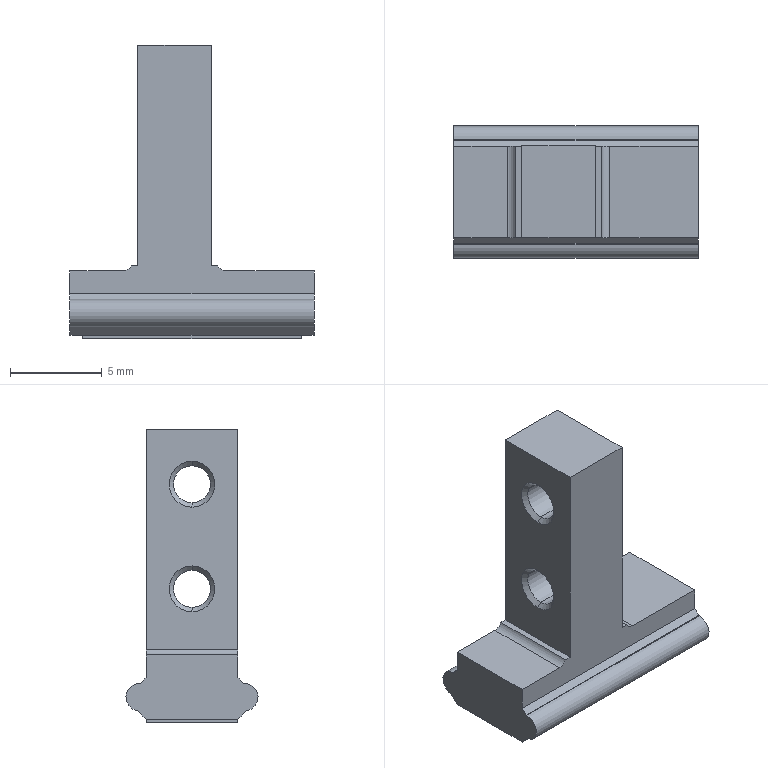Part | SolidWorks | features ICE 5, Chamfer 3, HoleWzd 2, Cut 1, Extrusion 1 | 1 solid | 43 faces | box 13.3 x 7.2 x 16 mm | volume 492.464 mm3 | plane 23 | cylinder 12 | cone 8 | commonest cylinder face diameters 1.5 x4 2.013 x4 1 x2 2.5 x2
STEP:
#1=CARTESIAN_POINT('',(-8.85,0.,3.));
#2=VERTEX_POINT('',#1);
#3=CARTESIAN_POINT('',(-11.35,0.,3.));
#4=VERTEX_POINT('',#3);
#5=CARTESIAN_POINT('',(-10.1,0.,3.));
#6=DIRECTION('',(0.,0.,-1.));
#7=DIRECTION('',(-1.,0.,0.));
#8=AXIS2_PLACEMENT_3D('',#5,#6,#7);
#9=CIRCLE('',#8,1.25);
#10=EDGE_CURVE('',#2,#4,#9,.T.);
#11=ORIENTED_EDGE('',*,*,#10,.F.);
#12=CARTESIAN_POINT('',(-8.85,0.,0.));
#13=VERTEX_POINT('',#12);
#14=CARTESIAN_POINT('',(-8.85,0.,3.));
#15=DIRECTION('',(0.,0.,-1.));
#16=VECTOR('',#15,1000.);
#17=LINE('',#14,#16);
#18=EDGE_CURVE('',#2,#13,#17,.T.);
#19=ORIENTED_EDGE('',*,*,#18,.T.);
#20=CARTESIAN_POINT('',(-11.35,0.,0.));
#21=VERTEX_POINT('',#20);
#22=CARTESIAN_POINT('',(-10.1,0.,0.));
#23=DIRECTION('',(0.,0.,-1.));
#24=DIRECTION('',(-1.,0.,0.));
#25=AXIS2_PLACEMENT_3D('',#22,#23,#24);
#26=CIRCLE('',#25,1.25);
#27=EDGE_CURVE('',#13,#21,#26,.T.);
#28=ORIENTED_EDGE('',*,*,#27,.T.);
#29=CARTESIAN_POINT('',(-11.35,0.,3.));
#30=DIRECTION('',(0.,0.,-1.));
#31=VECTOR('',#30,1000.);
#32=LINE('',#29,#31);
#33=EDGE_CURVE('',#4,#21,#32,.T.);
#34=ORIENTED_EDGE('',*,*,#33,.F.);
#35=EDGE_LOOP('',(#11,#19,#28,#34));
#36=FACE_OUTER_BOUND('',#35,.T.);
#37=CARTESIAN_POINT('',(-10.1,0.,3.));
#38=DIRECTION('',(0.,0.,-1.));
#39=DIRECTION('',(-1.,0.,0.));
#40=AXIS2_PLACEMENT_3D('',#37,#38,#39);
#41=CYLINDRICAL_SURFACE('',#40,1.25);
#42=ADVANCED_FACE('',(#36),#41,.F.);
#43=CARTESIAN_POINT('',(-13.357,0.,11.993));
#44=VERTEX_POINT('',#43);
#45=CARTESIAN_POINT('',(-13.357,0.,14.007));
#46=VERTEX_POINT('',#45);
#47=CARTESIAN_POINT('',(-13.357,0.,13.));
#48=DIRECTION('',(-1.,0.,0.));
#49=DIRECTION('',(0.,0.,-1.));
#50=AXIS2_PLACEMENT_3D('',#47,#48,#49);
#51=CIRCLE('',#50,1.007);
#52=EDGE_CURVE('',#44,#46,#51,.T.);
#53=ORIENTED_EDGE('',*,*,#52,.F.);
#54=CARTESIAN_POINT('',(-13.6,0.,11.75));
#55=VERTEX_POINT('',#54);
#56=CARTESIAN_POINT('',(-13.357,0.,11.993));
#57=DIRECTION('',(-0.7071,0.,-0.7071));
#58=VECTOR('',#57,1000.);
#59=LINE('',#56,#58);
#60=EDGE_CURVE('',#44,#55,#59,.T.);
#61=ORIENTED_EDGE('',*,*,#60,.T.);
#62=CARTESIAN_POINT('',(-13.6,0.,14.25));
#63=VERTEX_POINT('',#62);
#64=CARTESIAN_POINT('',(-13.6,0.,13.));
#65=DIRECTION('',(1.,0.,0.));
#66=DIRECTION('',(0.,0.,-1.));
#67=AXIS2_PLACEMENT_3D('',#64,#65,#66);
#68=CIRCLE('',#67,1.25);
#69=EDGE_CURVE('',#63,#55,#68,.T.);
#70=ORIENTED_EDGE('',*,*,#69,.F.);
#71=CARTESIAN_POINT('',(-13.357,0.,14.007));
#72=DIRECTION('',(-0.7071,0.,0.7071));
#73=VECTOR('',#72,1000.);
#74=LINE('',#71,#73);
#75=EDGE_CURVE('',#46,#63,#74,.T.);
#76=ORIENTED_EDGE('',*,*,#75,.F.);
#77=EDGE_LOOP('',(#53,#61,#70,#76));
#78=FACE_OUTER_BOUND('',#77,.T.);
#79=CARTESIAN_POINT('',(-13.357,0.,13.));
#80=DIRECTION('',(-1.,0.,0.));
#81=DIRECTION('',(0.,0.,1.));
#82=AXIS2_PLACEMENT_3D('',#79,#80,#81);
#83=CONICAL_SURFACE('',#82,1.007,0.7854);
#84=ADVANCED_FACE('',(#78),#83,.F.);
#85=CARTESIAN_POINT('',(-9.844,0.,14.007));
#86=VERTEX_POINT('',#85);
#87=CARTESIAN_POINT('',(-9.844,0.,11.993));
#88=VERTEX_POINT('',#87);
#89=CARTESIAN_POINT('',(-9.844,0.,13.));
#90=DIRECTION('',(1.,0.,0.));
#91=DIRECTION('',(0.,0.,1.));
#92=AXIS2_PLACEMENT_3D('',#89,#90,#91);
#93=CIRCLE('',#92,1.007);
#94=EDGE_CURVE('',#86,#88,#93,.T.);
#95=ORIENTED_EDGE('',*,*,#94,.F.);
#96=CARTESIAN_POINT('',(-9.6,0.,14.25));
#97=VERTEX_POINT('',#96);
#98=CARTESIAN_POINT('',(-9.6,0.,14.25));
#99=DIRECTION('',(0.7071,0.,0.7071));
#100=VECTOR('',#99,1000.);
#101=LINE('',#98,#100);
#102=EDGE_CURVE('',#86,#97,#101,.T.);
#103=ORIENTED_EDGE('',*,*,#102,.T.);
#104=CARTESIAN_POINT('',(-9.6,0.,11.75));
#105=VERTEX_POINT('',#104);
#106=CARTESIAN_POINT('',(-9.6,0.,13.));
#107=DIRECTION('',(-1.,0.,0.));
#108=DIRECTION('',(0.,0.,1.));
#109=AXIS2_PLACEMENT_3D('',#106,#107,#108);
#110=CIRCLE('',#109,1.25);
#111=EDGE_CURVE('',#105,#97,#110,.T.);
#112=ORIENTED_EDGE('',*,*,#111,.F.);
#113=CARTESIAN_POINT('',(-9.6,0.,11.75));
#114=DIRECTION('',(0.7071,0.,-0.7071));
#115=VECTOR('',#114,1000.);
#116=LINE('',#113,#115);
#117=EDGE_CURVE('',#88,#105,#116,.T.);
#118=ORIENTED_EDGE('',*,*,#117,.F.);
#119=EDGE_LOOP('',(#95,#103,#112,#118));
#120=FACE_OUTER_BOUND('',#119,.T.);
#121=CARTESIAN_POINT('',(-9.6,0.,13.));
#122=DIRECTION('',(1.,0.,0.));
#123=DIRECTION('',(0.,0.,-1.));
#124=AXIS2_PLACEMENT_3D('',#121,#122,#123);
#125=CONICAL_SURFACE('',#124,1.25,0.7854);
#126=ADVANCED_FACE('',(#120),#125,.F.);
#127=CARTESIAN_POINT('',(-9.843,0.,8.307));
#128=VERTEX_POINT('',#127);
#129=CARTESIAN_POINT('',(-9.843,0.,6.293));
#130=VERTEX_POINT('',#129);
#131=CARTESIAN_POINT('',(-9.843,0.,7.3));
#132=DIRECTION('',(1.,0.,0.));
#133=DIRECTION('',(0.,0.,1.));
#134=AXIS2_PLACEMENT_3D('',#131,#132,#133);
#135=CIRCLE('',#134,1.007);
#136=EDGE_CURVE('',#128,#130,#135,.T.);
#137=ORIENTED_EDGE('',*,*,#136,.F.);
#138=CARTESIAN_POINT('',(-9.6,0.,8.55));
#139=VERTEX_POINT('',#138);
#140=CARTESIAN_POINT('',(-9.843,0.,8.307));
#141=DIRECTION('',(0.7071,0.,0.7071));
#142=VECTOR('',#141,1000.);
#143=LINE('',#140,#142);
#144=EDGE_CURVE('',#128,#139,#143,.T.);
#145=ORIENTED_EDGE('',*,*,#144,.T.);
#146=CARTESIAN_POINT('',(-9.6,0.,6.05));
#147=VERTEX_POINT('',#146);
#148=CARTESIAN_POINT('',(-9.6,0.,7.3));
#149=DIRECTION('',(-1.,0.,0.));
#150=DIRECTION('',(0.,0.,1.));
#151=AXIS2_PLACEMENT_3D('',#148,#149,#150);
#152=CIRCLE('',#151,1.25);
#153=EDGE_CURVE('',#147,#139,#152,.T.);
#154=ORIENTED_EDGE('',*,*,#153,.F.);
#155=CARTESIAN_POINT('',(-9.843,0.,6.293));
#156=DIRECTION('',(0.7071,0.,-0.7071));
#157=VECTOR('',#156,1000.);
#158=LINE('',#155,#157);
#159=EDGE_CURVE('',#130,#147,#158,.T.);
#160=ORIENTED_EDGE('',*,*,#159,.F.);
#161=EDGE_LOOP('',(#137,#145,#154,#160));
#162=FACE_OUTER_BOUND('',#161,.T.);
#163=CARTESIAN_POINT('',(-9.843,0.,7.3));
#164=DIRECTION('',(1.,0.,0.));
#165=DIRECTION('',(0.,0.,-1.));
#166=AXIS2_PLACEMENT_3D('',#163,#164,#165);
#167=CONICAL_SURFACE('',#166,1.007,0.7854);
#168=ADVANCED_FACE('',(#162),#167,.F.);
#169=CARTESIAN_POINT('',(-13.357,0.,6.293));
#170=VERTEX_POINT('',#169);
#171=CARTESIAN_POINT('',(-13.357,0.,8.307));
#172=VERTEX_POINT('',#171);
#173=CARTESIAN_POINT('',(-13.357,0.,7.3));
#174=DIRECTION('',(-1.,0.,0.));
#175=DIRECTION('',(0.,0.,-1.));
#176=AXIS2_PLACEMENT_3D('',#173,#174,#175);
#177=CIRCLE('',#176,1.007);
#178=EDGE_CURVE('',#170,#172,#177,.T.);
#179=ORIENTED_EDGE('',*,*,#178,.F.);
#180=CARTESIAN_POINT('',(-13.6,0.,6.05));
#181=VERTEX_POINT('',#180);
#182=CARTESIAN_POINT('',(-13.6,0.,6.05));
#183=DIRECTION('',(-0.7071,0.,-0.7071));
#184=VECTOR('',#183,1000.);
#185=LINE('',#182,#184);
#186=EDGE_CURVE('',#170,#181,#185,.T.);
#187=ORIENTED_EDGE('',*,*,#186,.T.);
#188=CARTESIAN_POINT('',(-13.6,0.,8.55));
#189=VERTEX_POINT('',#188);
#190=CARTESIAN_POINT('',(-13.6,0.,7.3));
#191=DIRECTION('',(1.,0.,0.));
#192=DIRECTION('',(0.,0.,-1.));
#193=AXIS2_PLACEMENT_3D('',#190,#191,#192);
#194=CIRCLE('',#193,1.25);
#195=EDGE_CURVE('',#189,#181,#194,.T.);
#196=ORIENTED_EDGE('',*,*,#195,.F.);
#197=CARTESIAN_POINT('',(-13.6,0.,8.55));
#198=DIRECTION('',(-0.7071,0.,0.7071));
#199=VECTOR('',#198,1000.);
#200=LINE('',#197,#199);
#201=EDGE_CURVE('',#172,#189,#200,.T.);
#202=ORIENTED_EDGE('',*,*,#201,.F.);
#203=EDGE_LOOP('',(#179,#187,#196,#202));
#204=FACE_OUTER_BOUND('',#203,.T.);
#205=CARTESIAN_POINT('',(-13.6,0.,7.3));
#206=DIRECTION('',(-1.,0.,0.));
#207=DIRECTION('',(0.,0.,1.));
#208=AXIS2_PLACEMENT_3D('',#205,#206,#207);
#209=CONICAL_SURFACE('',#208,1.25,0.7854);
#210=ADVANCED_FACE('',(#204),#209,.F.);
#211=ORIENTED_EDGE('',*,*,#94,.T.);
#212=CARTESIAN_POINT('',(-13.6,0.,11.993));
#213=DIRECTION('',(-1.,0.,0.));
#214=VECTOR('',#213,1000.);
#215=LINE('',#212,#214);
#216=EDGE_CURVE('',#88,#44,#215,.T.);
#217=ORIENTED_EDGE('',*,*,#216,.T.);
#218=ORIENTED_EDGE('',*,*,#52,.T.);
#219=CARTESIAN_POINT('',(-13.6,0.,14.007));
#220=DIRECTION('',(-1.,0.,0.));
#221=VECTOR('',#220,1000.);
#222=LINE('',#219,#221);
#223=EDGE_CURVE('',#86,#46,#222,.T.);
#224=ORIENTED_EDGE('',*,*,#223,.F.);
#225=EDGE_LOOP('',(#211,#217,#218,#224));
#226=FACE_OUTER_BOUND('',#225,.T.);
#227=CARTESIAN_POINT('',(-13.6,0.,13.));
#228=DIRECTION('',(-1.,0.,0.));
#229=DIRECTION('',(0.,0.,1.));
#230=AXIS2_PLACEMENT_3D('',#227,#228,#229);
#231=CYLINDRICAL_SURFACE('',#230,1.007);
#232=ADVANCED_FACE('',(#226),#231,.F.);
#233=ORIENTED_EDGE('',*,*,#178,.T.);
#234=CARTESIAN_POINT('',(-9.6,0.,8.307));
#235=DIRECTION('',(1.,0.,0.));
#236=VECTOR('',#235,1000.);
#237=LINE('',#234,#236);
#238=EDGE_CURVE('',#172,#128,#237,.T.);
#239=ORIENTED_EDGE('',*,*,#238,.T.);
#240=ORIENTED_EDGE('',*,*,#136,.T.);
#241=CARTESIAN_POINT('',(-9.6,0.,6.293));
#242=DIRECTION('',(1.,0.,0.));
#243=VECTOR('',#242,1000.);
#244=LINE('',#241,#243);
#245=EDGE_CURVE('',#170,#130,#244,.T.);
#246=ORIENTED_EDGE('',*,*,#245,.F.);
#247=EDGE_LOOP('',(#233,#239,#240,#246));
#248=FACE_OUTER_BOUND('',#247,.T.);
#249=CARTESIAN_POINT('',(-9.6,0.,7.3));
#250=DIRECTION('',(1.,0.,0.));
#251=DIRECTION('',(0.,0.,-1.));
#252=AXIS2_PLACEMENT_3D('',#249,#250,#251);
#253=CYLINDRICAL_SURFACE('',#252,1.007);
#254=ADVANCED_FACE('',(#248),#253,.F.);
#255=CARTESIAN_POINT('',(-4.,2.806,2.149));
#256=VERTEX_POINT('',#255);
#257=CARTESIAN_POINT('',(-4.,2.85,2.15));
#258=VERTEX_POINT('',#257);
#259=CARTESIAN_POINT('',(-4.,2.85,1.4));
#260=DIRECTION('',(-1.,0.,0.));
#261=DIRECTION('',(0.,0.,1.));
#262=AXIS2_PLACEMENT_3D('',#259,#260,#261);
#263=CIRCLE('',#262,0.75);
#264=EDGE_CURVE('',#256,#258,#263,.T.);
#265=ORIENTED_EDGE('',*,*,#264,.T.);
#266=CARTESIAN_POINT('',(-17.3,2.85,2.15));
#267=VERTEX_POINT('',#266);
#268=CARTESIAN_POINT('',(-4.,2.85,2.15));
#269=DIRECTION('',(-1.,0.,0.));
#270=VECTOR('',#269,1000.);
#271=LINE('',#268,#270);
#272=EDGE_CURVE('',#258,#267,#271,.T.);
#273=ORIENTED_EDGE('',*,*,#272,.T.);
#274=CARTESIAN_POINT('',(-17.3,2.806,2.149));
#275=VERTEX_POINT('',#274);
#276=CARTESIAN_POINT('',(-17.3,2.85,1.4));
#277=DIRECTION('',(-1.,0.,0.));
#278=DIRECTION('',(0.,0.,1.));
#279=AXIS2_PLACEMENT_3D('',#276,#277,#278);
#280=CIRCLE('',#279,0.75);
#281=EDGE_CURVE('',#275,#267,#280,.T.);
#282=ORIENTED_EDGE('',*,*,#281,.F.);
#283=CARTESIAN_POINT('',(-4.,2.806,2.149));
#284=DIRECTION('',(1.,0.,0.));
#285=VECTOR('',#284,1000.);
#286=LINE('',#283,#285);
#287=EDGE_CURVE('',#275,#256,#286,.T.);
#288=ORIENTED_EDGE('',*,*,#287,.T.);
#289=EDGE_LOOP('',(#265,#273,#282,#288));
#290=FACE_OUTER_BOUND('',#289,.T.);
#291=CARTESIAN_POINT('',(-4.,2.85,1.4));
#292=DIRECTION('',(-1.,0.,0.));
#293=DIRECTION('',(0.,0.,1.));
#294=AXIS2_PLACEMENT_3D('',#291,#292,#293);
#295=CYLINDRICAL_SURFACE('',#294,0.75);
#296=ADVANCED_FACE('',(#290),#295,.T.);
#297=CARTESIAN_POINT('',(-4.,-2.958,0.6578));
#298=VERTEX_POINT('',#297);
#299=CARTESIAN_POINT('',(-4.,-2.85,2.15));
#300=VERTEX_POINT('',#299);
#301=CARTESIAN_POINT('',(-4.,-2.85,1.4));
#302=DIRECTION('',(-1.,0.,0.));
#303=DIRECTION('',(0.,0.,1.));
#304=AXIS2_PLACEMENT_3D('',#301,#302,#303);
#305=CIRCLE('',#304,0.75);
#306=EDGE_CURVE('',#298,#300,#305,.T.);
#307=ORIENTED_EDGE('',*,*,#306,.T.);
#308=CARTESIAN_POINT('',(-17.3,-2.85,2.15));
#309=VERTEX_POINT('',#308);
#310=CARTESIAN_POINT('',(-4.,-2.85,2.15));
#311=DIRECTION('',(-1.,0.,0.));
#312=VECTOR('',#311,1000.);
#313=LINE('',#310,#312);
#314=EDGE_CURVE('',#300,#309,#313,.T.);
#315=ORIENTED_EDGE('',*,*,#314,.T.);
#316=CARTESIAN_POINT('',(-17.3,-2.958,0.6578));
#317=VERTEX_POINT('',#316);
#318=CARTESIAN_POINT('',(-17.3,-2.85,1.4));
#319=DIRECTION('',(-1.,0.,0.));
#320=DIRECTION('',(0.,0.,1.));
#321=AXIS2_PLACEMENT_3D('',#318,#319,#320);
#322=CIRCLE('',#321,0.75);
#323=EDGE_CURVE('',#317,#309,#322,.T.);
#324=ORIENTED_EDGE('',*,*,#323,.F.);
#325=CARTESIAN_POINT('',(-4.,-2.958,0.6578));
#326=DIRECTION('',(-1.,0.,0.));
#327=VECTOR('',#326,1000.);
#328=LINE('',#325,#327);
#329=EDGE_CURVE('',#298,#317,#328,.T.);
#330=ORIENTED_EDGE('',*,*,#329,.F.);
#331=EDGE_LOOP('',(#307,#315,#324,#330));
#332=FACE_OUTER_BOUND('',#331,.T.);
#333=CARTESIAN_POINT('',(-4.,-2.85,1.4));
#334=DIRECTION('',(-1.,0.,0.));
#335=DIRECTION('',(0.,0.,1.));
#336=AXIS2_PLACEMENT_3D('',#333,#334,#335);
#337=CYLINDRICAL_SURFACE('',#336,0.75);
#338=ADVANCED_FACE('',(#332),#337,.T.);
#339=CARTESIAN_POINT('',(-16.6,-2.5,0.2));
#340=VERTEX_POINT('',#339);
#341=CARTESIAN_POINT('',(-16.6,2.5,0.2));
#342=VERTEX_POINT('',#341);
#343=CARTESIAN_POINT('',(-16.6,2.5,0.2));
#344=DIRECTION('',(0.,1.,0.));
#345=VECTOR('',#344,1000.);
#346=LINE('',#343,#345);
#347=EDGE_CURVE('',#340,#342,#346,.T.);
#348=ORIENTED_EDGE('',*,*,#347,.F.);
#349=CARTESIAN_POINT('',(-17.3,-2.5,0.2));
#350=VERTEX_POINT('',#349);
#351=CARTESIAN_POINT('',(-4.,-2.5,0.2));
#352=DIRECTION('',(-1.,0.,0.));
#353=VECTOR('',#352,1000.);
#354=LINE('',#351,#353);
#355=EDGE_CURVE('',#340,#350,#354,.T.);
#356=ORIENTED_EDGE('',*,*,#355,.T.);
#357=CARTESIAN_POINT('',(-17.3,2.5,0.2));
#358=VERTEX_POINT('',#357);
#359=CARTESIAN_POINT('',(-17.3,2.5,0.2));
#360=DIRECTION('',(0.,-1.,0.));
#361=VECTOR('',#360,1000.);
#362=LINE('',#359,#361);
#363=EDGE_CURVE('',#358,#350,#362,.T.);
#364=ORIENTED_EDGE('',*,*,#363,.F.);
#365=CARTESIAN_POINT('',(-4.,2.5,0.2));
#366=DIRECTION('',(-1.,0.,0.));
#367=VECTOR('',#366,1000.);
#368=LINE('',#365,#367);
#369=EDGE_CURVE('',#342,#358,#368,.T.);
#370=ORIENTED_EDGE('',*,*,#369,.F.);
#371=EDGE_LOOP('',(#348,#356,#364,#370));
#372=FACE_OUTER_BOUND('',#371,.T.);
#373=CARTESIAN_POINT('',(-4.,2.5,0.2));
#374=DIRECTION('',(0.,0.,-1.));
#375=DIRECTION('',(-1.,0.,0.));
#376=AXIS2_PLACEMENT_3D('',#373,#374,#375);
#377=PLANE('',#376);
#378=ADVANCED_FACE('',(#372),#377,.T.);
#379=CARTESIAN_POINT('',(-13.6,-2.5,16.));
#380=VERTEX_POINT('',#379);
#381=CARTESIAN_POINT('',(-13.6,2.5,16.));
#382=VERTEX_POINT('',#381);
#383=CARTESIAN_POINT('',(-13.6,-3.6,16.));
#384=DIRECTION('',(0.,1.,0.));
#385=VECTOR('',#384,1000.);
#386=LINE('',#383,#385);
#387=EDGE_CURVE('',#380,#382,#386,.T.);
#388=ORIENTED_EDGE('',*,*,#387,.F.);
#389=CARTESIAN_POINT('',(-9.6,-2.5,16.));
#390=VERTEX_POINT('',#389);
#391=CARTESIAN_POINT('',(-4.,-2.5,16.));
#392=DIRECTION('',(-1.,0.,0.));
#393=VECTOR('',#392,1000.);
#394=LINE('',#391,#393);
#395=EDGE_CURVE('',#390,#380,#394,.T.);
#396=ORIENTED_EDGE('',*,*,#395,.F.);
#397=CARTESIAN_POINT('',(-9.6,2.5,16.));
#398=VERTEX_POINT('',#397);
#399=CARTESIAN_POINT('',(-9.6,-3.6,16.));
#400=DIRECTION('',(0.,1.,0.));
#401=VECTOR('',#400,1000.);
#402=LINE('',#399,#401);
#403=EDGE_CURVE('',#390,#398,#402,.T.);
#404=ORIENTED_EDGE('',*,*,#403,.T.);
#405=CARTESIAN_POINT('',(-4.,2.5,16.));
#406=DIRECTION('',(-1.,0.,0.));
#407=VECTOR('',#406,1000.);
#408=LINE('',#405,#407);
#409=EDGE_CURVE('',#398,#382,#408,.T.);
#410=ORIENTED_EDGE('',*,*,#409,.T.);
#411=EDGE_LOOP('',(#388,#396,#404,#410));
#412=FACE_OUTER_BOUND('',#411,.T.);
#413=CARTESIAN_POINT('',(-4.,-2.5,16.));
#414=DIRECTION('',(0.,0.,1.));
#415=DIRECTION('',(1.,0.,0.));
#416=AXIS2_PLACEMENT_3D('',#413,#414,#415);
#417=PLANE('',#416);
#418=ADVANCED_FACE('',(#412),#417,.T.);
#419=CARTESIAN_POINT('',(-17.3,-2.5,2.455));
#420=VERTEX_POINT('',#419);
#421=CARTESIAN_POINT('',(-17.3,-2.5,3.7));
#422=VERTEX_POINT('',#421);
#423=CARTESIAN_POINT('',(-17.3,-2.5,2.063));
#424=DIRECTION('',(0.,0.,1.));
#425=VECTOR('',#424,1000.);
#426=LINE('',#423,#425);
#427=EDGE_CURVE('',#420,#422,#426,.T.);
#428=ORIENTED_EDGE('',*,*,#427,.F.);
#429=CARTESIAN_POINT('',(-4.,-2.5,2.455));
#430=VERTEX_POINT('',#429);
#431=CARTESIAN_POINT('',(-4.,-2.5,2.455));
#432=DIRECTION('',(1.,0.,0.));
#433=VECTOR('',#432,1000.);
#434=LINE('',#431,#433);
#435=EDGE_CURVE('',#420,#430,#434,.T.);
#436=ORIENTED_EDGE('',*,*,#435,.T.);
#437=CARTESIAN_POINT('',(-4.,-2.5,3.7));
#438=VERTEX_POINT('',#437);
#439=CARTESIAN_POINT('',(-4.,-2.5,2.063));
#440=DIRECTION('',(0.,0.,1.));
#441=VECTOR('',#440,1000.);
#442=LINE('',#439,#441);
#443=EDGE_CURVE('',#430,#438,#442,.T.);
#444=ORIENTED_EDGE('',*,*,#443,.T.);
#445=CARTESIAN_POINT('',(-8.8,-2.5,3.7));
#446=VERTEX_POINT('',#445);
#447=CARTESIAN_POINT('',(-4.,-2.5,3.7));
#448=DIRECTION('',(1.,0.,0.));
#449=VECTOR('',#448,1000.);
#450=LINE('',#447,#449);
#451=EDGE_CURVE('',#446,#438,#450,.T.);
#452=ORIENTED_EDGE('',*,*,#451,.F.);
#453=CARTESIAN_POINT('',(-9.258,-2.5,4.));
#454=VERTEX_POINT('',#453);
#455=CARTESIAN_POINT('',(-8.8,-2.5,4.2));
#456=DIRECTION('',(0.,-1.,0.));
#457=DIRECTION('',(0.,0.,-1.));
#458=AXIS2_PLACEMENT_3D('',#455,#456,#457);
#459=CIRCLE('',#458,0.5);
#460=EDGE_CURVE('',#454,#446,#459,.T.);
#461=ORIENTED_EDGE('',*,*,#460,.F.);
#462=CARTESIAN_POINT('',(-9.6,-2.5,4.));
#463=VERTEX_POINT('',#462);
#464=CARTESIAN_POINT('',(-4.,-2.5,4.));
#465=DIRECTION('',(1.,0.,0.));
#466=VECTOR('',#465,1000.);
#467=LINE('',#464,#466);
#468=EDGE_CURVE('',#463,#454,#467,.T.);
#469=ORIENTED_EDGE('',*,*,#468,.F.);
#470=CARTESIAN_POINT('',(-9.6,-2.5,2.063));
#471=DIRECTION('',(0.,0.,-1.));
#472=VECTOR('',#471,1000.);
#473=LINE('',#470,#472);
#474=EDGE_CURVE('',#390,#463,#473,.T.);
#475=ORIENTED_EDGE('',*,*,#474,.F.);
#476=ORIENTED_EDGE('',*,*,#395,.T.);
#477=CARTESIAN_POINT('',(-13.6,-2.5,4.));
#478=VERTEX_POINT('',#477);
#479=CARTESIAN_POINT('',(-13.6,-2.5,2.063));
#480=DIRECTION('',(0.,0.,1.));
#481=VECTOR('',#480,1000.);
#482=LINE('',#479,#481);
#483=EDGE_CURVE('',#478,#380,#482,.T.);
#484=ORIENTED_EDGE('',*,*,#483,.F.);
#485=CARTESIAN_POINT('',(-13.942,-2.5,4.));
#486=VERTEX_POINT('',#485);
#487=CARTESIAN_POINT('',(-4.,-2.5,4.));
#488=DIRECTION('',(1.,0.,0.));
#489=VECTOR('',#488,1000.);
#490=LINE('',#487,#489);
#491=EDGE_CURVE('',#486,#478,#490,.T.);
#492=ORIENTED_EDGE('',*,*,#491,.F.);
#493=CARTESIAN_POINT('',(-14.4,-2.5,3.7));
#494=VERTEX_POINT('',#493);
#495=CARTESIAN_POINT('',(-14.4,-2.5,4.2));
#496=DIRECTION('',(0.,-1.,0.));
#497=DIRECTION('',(0.,0.,-1.));
#498=AXIS2_PLACEMENT_3D('',#495,#496,#497);
#499=CIRCLE('',#498,0.5);
#500=EDGE_CURVE('',#494,#486,#499,.T.);
#501=ORIENTED_EDGE('',*,*,#500,.F.);
#502=CARTESIAN_POINT('',(-4.,-2.5,3.7));
#503=DIRECTION('',(1.,0.,0.));
#504=VECTOR('',#503,1000.);
#505=LINE('',#502,#504);
#506=EDGE_CURVE('',#422,#494,#505,.T.);
#507=ORIENTED_EDGE('',*,*,#506,.F.);
#508=EDGE_LOOP('',(#428,#436,#444,#452,#461,#469,#475,#476,#484,#492,#501,#507));
#509=FACE_OUTER_BOUND('',#508,.T.);
#510=CARTESIAN_POINT('',(-4.,-2.5,2.063));
#511=DIRECTION('',(0.,-1.,0.));
#512=DIRECTION('',(0.,0.,-1.));
#513=AXIS2_PLACEMENT_3D('',#510,#511,#512);
#514=PLANE('',#513);
#515=ADVANCED_FACE('',(#509),#514,.T.);
#516=ORIENTED_EDGE('',*,*,#314,.F.);
#517=CARTESIAN_POINT('',(-4.,-2.806,2.149));
#518=VERTEX_POINT('',#517);
#519=CARTESIAN_POINT('',(-4.,-2.85,1.4));
#520=DIRECTION('',(-1.,0.,0.));
#521=DIRECTION('',(0.,0.,1.));
#522=AXIS2_PLACEMENT_3D('',#519,#520,#521);
#523=CIRCLE('',#522,0.75);
#524=EDGE_CURVE('',#300,#518,#523,.T.);
#525=ORIENTED_EDGE('',*,*,#524,.T.);
#526=CARTESIAN_POINT('',(-17.3,-2.806,2.149));
#527=VERTEX_POINT('',#526);
#528=CARTESIAN_POINT('',(-4.,-2.806,2.149));
#529=DIRECTION('',(-1.,0.,0.));
#530=VECTOR('',#529,1000.);
#531=LINE('',#528,#530);
#532=EDGE_CURVE('',#518,#527,#531,.T.);
#533=ORIENTED_EDGE('',*,*,#532,.T.);
#534=CARTESIAN_POINT('',(-17.3,-2.85,1.4));
#535=DIRECTION('',(-1.,0.,0.));
#536=DIRECTION('',(0.,0.,1.));
#537=AXIS2_PLACEMENT_3D('',#534,#535,#536);
#538=CIRCLE('',#537,0.75);
#539=EDGE_CURVE('',#309,#527,#538,.T.);
#540=ORIENTED_EDGE('',*,*,#539,.F.);
#541=EDGE_LOOP('',(#516,#525,#533,#540));
#542=FACE_OUTER_BOUND('',#541,.T.);
#543=CARTESIAN_POINT('',(-4.,-2.85,1.4));
#544=DIRECTION('',(-1.,0.,0.));
#545=DIRECTION('',(0.,0.,1.));
#546=AXIS2_PLACEMENT_3D('',#543,#544,#545);
#547=CYLINDRICAL_SURFACE('',#546,0.75);
#548=ADVANCED_FACE('',(#542),#547,.T.);
#549=CARTESIAN_POINT('',(-17.3,-2.5,0.2));
#550=DIRECTION('',(0.,-0.7071,0.7071));
#551=VECTOR('',#550,1000.);
#552=LINE('',#549,#551);
#553=EDGE_CURVE('',#350,#317,#552,.T.);
#554=ORIENTED_EDGE('',*,*,#553,.F.);
#555=ORIENTED_EDGE('',*,*,#355,.F.);
#556=CARTESIAN_POINT('',(-4.7,-2.5,0.2));
#557=VERTEX_POINT('',#556);
#558=CARTESIAN_POINT('',(-16.6,-2.5,0.2));
#559=DIRECTION('',(-1.,0.,0.));
#560=VECTOR('',#559,1000.);
#561=LINE('',#558,#560);
#562=EDGE_CURVE('',#557,#340,#561,.T.);
#563=ORIENTED_EDGE('',*,*,#562,.F.);
#564=CARTESIAN_POINT('',(-4.,-2.5,0.2));
#565=VERTEX_POINT('',#564);
#566=CARTESIAN_POINT('',(-4.,-2.5,0.2));
#567=DIRECTION('',(-1.,0.,0.));
#568=VECTOR('',#567,1000.);
#569=LINE('',#566,#568);
#570=EDGE_CURVE('',#565,#557,#569,.T.);
#571=ORIENTED_EDGE('',*,*,#570,.F.);
#572=CARTESIAN_POINT('',(-4.,-2.5,0.2));
#573=DIRECTION('',(0.,-0.7071,0.7071));
#574=VECTOR('',#573,1000.);
#575=LINE('',#572,#574);
#576=EDGE_CURVE('',#565,#298,#575,.T.);
#577=ORIENTED_EDGE('',*,*,#576,.T.);
#578=ORIENTED_EDGE('',*,*,#329,.T.);
#579=EDGE_LOOP('',(#554,#555,#563,#571,#577,#578));
#580=FACE_OUTER_BOUND('',#579,.T.);
#581=CARTESIAN_POINT('',(-4.,-2.5,0.2));
#582=DIRECTION('',(0.,-0.7071,-0.7071));
#583=DIRECTION('',(0.,0.7071,-0.7071));
#584=AXIS2_PLACEMENT_3D('',#581,#582,#583);
#585=PLANE('',#584);
#586=ADVANCED_FACE('',(#580),#585,.T.);
#587=CARTESIAN_POINT('',(-4.7,2.5,0.2));
#588=VERTEX_POINT('',#587);
#589=CARTESIAN_POINT('',(-4.7,-2.5,0.2));
#590=DIRECTION('',(0.,-1.,0.));
#591=VECTOR('',#590,1000.);
#592=LINE('',#589,#591);
#593=EDGE_CURVE('',#588,#557,#592,.T.);
#594=ORIENTED_EDGE('',*,*,#593,.F.);
#595=CARTESIAN_POINT('',(-4.,2.5,0.2));
#596=VERTEX_POINT('',#595);
#597=CARTESIAN_POINT('',(-4.,2.5,0.2));
#598=DIRECTION('',(-1.,0.,0.));
#599=VECTOR('',#598,1000.);
#600=LINE('',#597,#599);
#601=EDGE_CURVE('',#596,#588,#600,.T.);
#602=ORIENTED_EDGE('',*,*,#601,.F.);
#603=CARTESIAN_POINT('',(-4.,2.5,0.2));
#604=DIRECTION('',(0.,-1.,0.));
#605=VECTOR('',#604,1000.);
#606=LINE('',#603,#605);
#607=EDGE_CURVE('',#596,#565,#606,.T.);
#608=ORIENTED_EDGE('',*,*,#607,.T.);
#609=ORIENTED_EDGE('',*,*,#570,.T.);
#610=EDGE_LOOP('',(#594,#602,#608,#609));
#611=FACE_OUTER_BOUND('',#610,.T.);
#612=CARTESIAN_POINT('',(-4.,2.5,0.2));
#613=DIRECTION('',(0.,0.,-1.));
#614=DIRECTION('',(-1.,0.,0.));
#615=AXIS2_PLACEMENT_3D('',#612,#613,#614);
#616=PLANE('',#615);
#617=ADVANCED_FACE('',(#611),#616,.T.);
#618=CARTESIAN_POINT('',(-17.3,2.958,0.6578));
#619=VERTEX_POINT('',#618);
#620=CARTESIAN_POINT('',(-17.3,2.958,0.6578));
#621=DIRECTION('',(0.,-0.7071,-0.7071));
#622=VECTOR('',#621,1000.);
#623=LINE('',#620,#622);
#624=EDGE_CURVE('',#619,#358,#623,.T.);
#625=ORIENTED_EDGE('',*,*,#624,.F.);
#626=CARTESIAN_POINT('',(-4.,2.958,0.6578));
#627=VERTEX_POINT('',#626);
#628=CARTESIAN_POINT('',(-4.,2.958,0.6578));
#629=DIRECTION('',(-1.,0.,0.));
#630=VECTOR('',#629,1000.);
#631=LINE('',#628,#630);
#632=EDGE_CURVE('',#627,#619,#631,.T.);
#633=ORIENTED_EDGE('',*,*,#632,.F.);
#634=CARTESIAN_POINT('',(-4.,2.958,0.6578));
#635=DIRECTION('',(0.,-0.7071,-0.7071));
#636=VECTOR('',#635,1000.);
#637=LINE('',#634,#636);
#638=EDGE_CURVE('',#627,#596,#637,.T.);
#639=ORIENTED_EDGE('',*,*,#638,.T.);
#640=ORIENTED_EDGE('',*,*,#601,.T.);
#641=CARTESIAN_POINT('',(-4.7,2.5,0.2));
#642=DIRECTION('',(1.,0.,0.));
#643=VECTOR('',#642,1000.);
#644=LINE('',#641,#643);
#645=EDGE_CURVE('',#342,#588,#644,.T.);
#646=ORIENTED_EDGE('',*,*,#645,.F.);
#647=ORIENTED_EDGE('',*,*,#369,.T.);
#648=EDGE_LOOP('',(#625,#633,#639,#640,#646,#647));
#649=FACE_OUTER_BOUND('',#648,.T.);
#650=CARTESIAN_POINT('',(-4.,2.958,0.6578));
#651=DIRECTION('',(0.,0.7071,-0.7071));
#652=DIRECTION('',(0.,0.7071,0.7071));
#653=AXIS2_PLACEMENT_3D('',#650,#651,#652);
#654=PLANE('',#653);
#655=ADVANCED_FACE('',(#649),#654,.T.);
#656=ORIENTED_EDGE('',*,*,#272,.F.);
#657=CARTESIAN_POINT('',(-4.,2.85,1.4));
#658=DIRECTION('',(-1.,0.,0.));
#659=DIRECTION('',(0.,0.,1.));
#660=AXIS2_PLACEMENT_3D('',#657,#658,#659);
#661=CIRCLE('',#660,0.75);
#662=EDGE_CURVE('',#258,#627,#661,.T.);
#663=ORIENTED_EDGE('',*,*,#662,.T.);
#664=ORIENTED_EDGE('',*,*,#632,.T.);
#665=CARTESIAN_POINT('',(-17.3,2.85,1.4));
#666=DIRECTION('',(-1.,0.,0.));
#667=DIRECTION('',(0.,0.,1.));
#668=AXIS2_PLACEMENT_3D('',#665,#666,#667);
#669=CIRCLE('',#668,0.75);
#670=EDGE_CURVE('',#267,#619,#669,.T.);
#671=ORIENTED_EDGE('',*,*,#670,.F.);
#672=EDGE_LOOP('',(#656,#663,#664,#671));
#673=FACE_OUTER_BOUND('',#672,.T.);
#674=CARTESIAN_POINT('',(-4.,2.85,1.4));
#675=DIRECTION('',(-1.,0.,0.));
#676=DIRECTION('',(0.,0.,1.));
#677=AXIS2_PLACEMENT_3D('',#674,#675,#676);
#678=CYLINDRICAL_SURFACE('',#677,0.75);
#679=ADVANCED_FACE('',(#673),#678,.T.);
#680=CARTESIAN_POINT('',(-4.,2.5,3.7));
#681=VERTEX_POINT('',#680);
#682=CARTESIAN_POINT('',(-4.,2.5,2.455));
#683=VERTEX_POINT('',#682);
#684=CARTESIAN_POINT('',(-4.,2.5,16.));
#685=DIRECTION('',(0.,0.,-1.));
#686=VECTOR('',#685,1000.);
#687=LINE('',#684,#686);
#688=EDGE_CURVE('',#681,#683,#687,.T.);
#689=ORIENTED_EDGE('',*,*,#688,.T.);
#690=CARTESIAN_POINT('',(-17.3,2.5,2.455));
#691=VERTEX_POINT('',#690);
#692=CARTESIAN_POINT('',(-17.3,2.5,2.455));
#693=DIRECTION('',(-1.,0.,0.));
#694=VECTOR('',#693,1000.);
#695=LINE('',#692,#694);
#696=EDGE_CURVE('',#683,#691,#695,.T.);
#697=ORIENTED_EDGE('',*,*,#696,.T.);
#698=CARTESIAN_POINT('',(-17.3,2.5,3.7));
#699=VERTEX_POINT('',#698);
#700=CARTESIAN_POINT('',(-17.3,2.5,16.));
#701=DIRECTION('',(0.,0.,-1.));
#702=VECTOR('',#701,1000.);
#703=LINE('',#700,#702);
#704=EDGE_CURVE('',#699,#691,#703,.T.);
#705=ORIENTED_EDGE('',*,*,#704,.F.);
#706=CARTESIAN_POINT('',(-14.4,2.5,3.7));
#707=VERTEX_POINT('',#706);
#708=CARTESIAN_POINT('',(-14.4,2.5,3.7));
#709=DIRECTION('',(-1.,0.,0.));
#710=VECTOR('',#709,1000.);
#711=LINE('',#708,#710);
#712=EDGE_CURVE('',#707,#699,#711,.T.);
#713=ORIENTED_EDGE('',*,*,#712,.F.);
#714=CARTESIAN_POINT('',(-13.942,2.5,4.));
#715=VERTEX_POINT('',#714);
#716=CARTESIAN_POINT('',(-14.4,2.5,4.2));
#717=DIRECTION('',(0.,1.,0.));
#718=DIRECTION('',(0.,0.,1.));
#719=AXIS2_PLACEMENT_3D('',#716,#717,#718);
#720=CIRCLE('',#719,0.5);
#721=EDGE_CURVE('',#715,#707,#720,.T.);
#722=ORIENTED_EDGE('',*,*,#721,.F.);
#723=CARTESIAN_POINT('',(-13.6,2.5,4.));
#724=VERTEX_POINT('',#723);
#725=CARTESIAN_POINT('',(-13.6,2.5,4.));
#726=DIRECTION('',(-1.,0.,0.));
#727=VECTOR('',#726,1000.);
#728=LINE('',#725,#727);
#729=EDGE_CURVE('',#724,#715,#728,.T.);
#730=ORIENTED_EDGE('',*,*,#729,.F.);
#731=CARTESIAN_POINT('',(-13.6,2.5,16.));
#732=DIRECTION('',(0.,0.,-1.));
#733=VECTOR('',#732,1000.);
#734=LINE('',#731,#733);
#735=EDGE_CURVE('',#382,#724,#734,.T.);
#736=ORIENTED_EDGE('',*,*,#735,.F.);
#737=ORIENTED_EDGE('',*,*,#409,.F.);
#738=CARTESIAN_POINT('',(-9.6,2.5,4.));
#739=VERTEX_POINT('',#738);
#740=CARTESIAN_POINT('',(-9.6,2.5,4.));
#741=DIRECTION('',(0.,0.,1.));
#742=VECTOR('',#741,1000.);
#743=LINE('',#740,#742);
#744=EDGE_CURVE('',#739,#398,#743,.T.);
#745=ORIENTED_EDGE('',*,*,#744,.F.);
#746=CARTESIAN_POINT('',(-9.258,2.5,4.));
#747=VERTEX_POINT('',#746);
#748=CARTESIAN_POINT('',(-4.,2.5,4.));
#749=DIRECTION('',(-1.,0.,0.));
#750=VECTOR('',#749,1000.);
#751=LINE('',#748,#750);
#752=EDGE_CURVE('',#747,#739,#751,.T.);
#753=ORIENTED_EDGE('',*,*,#752,.F.);
#754=CARTESIAN_POINT('',(-8.8,2.5,3.7));
#755=VERTEX_POINT('',#754);
#756=CARTESIAN_POINT('',(-8.8,2.5,4.2));
#757=DIRECTION('',(0.,1.,0.));
#758=DIRECTION('',(0.,0.,1.));
#759=AXIS2_PLACEMENT_3D('',#756,#757,#758);
#760=CIRCLE('',#759,0.5);
#761=EDGE_CURVE('',#755,#747,#760,.T.);
#762=ORIENTED_EDGE('',*,*,#761,.F.);
#763=CARTESIAN_POINT('',(-4.,2.5,3.7));
#764=DIRECTION('',(-1.,0.,0.));
#765=VECTOR('',#764,1000.);
#766=LINE('',#763,#765);
#767=EDGE_CURVE('',#681,#755,#766,.T.);
#768=ORIENTED_EDGE('',*,*,#767,.F.);
#769=EDGE_LOOP('',(#689,#697,#705,#713,#722,#730,#736,#737,#745,#753,#762,#768));
#770=FACE_OUTER_BOUND('',#769,.T.);
#771=CARTESIAN_POINT('',(-4.,2.5,16.));
#772=DIRECTION('',(0.,1.,0.));
#773=DIRECTION('',(0.,0.,1.));
#774=AXIS2_PLACEMENT_3D('',#771,#772,#773);
#775=PLANE('',#774);
#776=ADVANCED_FACE('',(#770),#775,.T.);
#777=ORIENTED_EDGE('',*,*,#688,.F.);
#778=CARTESIAN_POINT('',(-4.,-3.6,3.7));
#779=DIRECTION('',(0.,1.,0.));
#780=VECTOR('',#779,1000.);
#781=LINE('',#778,#780);
#782=EDGE_CURVE('',#438,#681,#781,.T.);
#783=ORIENTED_EDGE('',*,*,#782,.F.);
#784=ORIENTED_EDGE('',*,*,#443,.F.);
#785=CARTESIAN_POINT('',(-4.,-0.3523,4.602));
#786=DIRECTION('',(0.,-0.7071,-0.7071));
#787=VECTOR('',#786,1000.);
#788=LINE('',#785,#787);
#789=EDGE_CURVE('',#430,#518,#788,.T.);
#790=ORIENTED_EDGE('',*,*,#789,.T.);
#791=ORIENTED_EDGE('',*,*,#524,.F.);
#792=ORIENTED_EDGE('',*,*,#306,.F.);
#793=ORIENTED_EDGE('',*,*,#576,.F.);
#794=ORIENTED_EDGE('',*,*,#607,.F.);
#795=ORIENTED_EDGE('',*,*,#638,.F.);
#796=ORIENTED_EDGE('',*,*,#662,.F.);
#797=ORIENTED_EDGE('',*,*,#264,.F.);
#798=CARTESIAN_POINT('',(-4.,3.202,1.752));
#799=DIRECTION('',(0.,-0.7071,0.7071));
#800=VECTOR('',#799,1000.);
#801=LINE('',#798,#800);
#802=EDGE_CURVE('',#256,#683,#801,.T.);
#803=ORIENTED_EDGE('',*,*,#802,.T.);
#804=EDGE_LOOP('',(#777,#783,#784,#790,#791,#792,#793,#794,#795,#796,#797,#803));
#805=FACE_OUTER_BOUND('',#804,.T.);
#806=CARTESIAN_POINT('',(-4.,2.85,1.4));
#807=DIRECTION('',(-1.,0.,0.));
#808=DIRECTION('',(0.,0.,1.));
#809=AXIS2_PLACEMENT_3D('',#806,#807,#808);
#810=PLANE('',#809);
#811=ADVANCED_FACE('',(#805),#810,.F.);
#812=CARTESIAN_POINT('',(-17.3,-3.6,3.7));
#813=DIRECTION('',(0.,1.,0.));
#814=VECTOR('',#813,1000.);
#815=LINE('',#812,#814);
#816=EDGE_CURVE('',#422,#699,#815,.T.);
#817=ORIENTED_EDGE('',*,*,#816,.T.);
#818=ORIENTED_EDGE('',*,*,#704,.T.);
#819=CARTESIAN_POINT('',(-17.3,2.5,2.455));
#820=DIRECTION('',(0.,0.7071,-0.7071));
#821=VECTOR('',#820,1000.);
#822=LINE('',#819,#821);
#823=EDGE_CURVE('',#691,#275,#822,.T.);
#824=ORIENTED_EDGE('',*,*,#823,.T.);
#825=ORIENTED_EDGE('',*,*,#281,.T.);
#826=ORIENTED_EDGE('',*,*,#670,.T.);
#827=ORIENTED_EDGE('',*,*,#624,.T.);
#828=ORIENTED_EDGE('',*,*,#363,.T.);
#829=ORIENTED_EDGE('',*,*,#553,.T.);
#830=ORIENTED_EDGE('',*,*,#323,.T.);
#831=ORIENTED_EDGE('',*,*,#539,.T.);
#832=CARTESIAN_POINT('',(-17.3,-2.806,2.149));
#833=DIRECTION('',(0.,0.7071,0.7071));
#834=VECTOR('',#833,1000.);
#835=LINE('',#832,#834);
#836=EDGE_CURVE('',#527,#420,#835,.T.);
#837=ORIENTED_EDGE('',*,*,#836,.T.);
#838=ORIENTED_EDGE('',*,*,#427,.T.);
#839=EDGE_LOOP('',(#817,#818,#824,#825,#826,#827,#828,#829,#830,#831,#837,#838));
#840=FACE_OUTER_BOUND('',#839,.T.);
#841=CARTESIAN_POINT('',(-17.3,2.85,1.4));
#842=DIRECTION('',(-1.,0.,0.));
#843=DIRECTION('',(0.,0.,1.));
#844=AXIS2_PLACEMENT_3D('',#841,#842,#843);
#845=PLANE('',#844);
#846=ADVANCED_FACE('',(#840),#845,.T.);
#847=ORIENTED_EDGE('',*,*,#347,.T.);
#848=CARTESIAN_POINT('',(-16.6,2.5,0.));
#849=VERTEX_POINT('',#848);
#850=CARTESIAN_POINT('',(-16.6,2.5,0.));
#851=DIRECTION('',(0.,0.,1.));
#852=VECTOR('',#851,1000.);
#853=LINE('',#850,#852);
#854=EDGE_CURVE('',#849,#342,#853,.T.);
#855=ORIENTED_EDGE('',*,*,#854,.F.);
#856=CARTESIAN_POINT('',(-16.6,-2.5,0.));
#857=VERTEX_POINT('',#856);
#858=CARTESIAN_POINT('',(-16.6,2.5,0.));
#859=DIRECTION('',(0.,1.,0.));
#860=VECTOR('',#859,1000.);
#861=LINE('',#858,#860);
#862=EDGE_CURVE('',#857,#849,#861,.T.);
#863=ORIENTED_EDGE('',*,*,#862,.F.);
#864=CARTESIAN_POINT('',(-16.6,-2.5,0.));
#865=DIRECTION('',(0.,0.,1.));
#866=VECTOR('',#865,1000.);
#867=LINE('',#864,#866);
#868=EDGE_CURVE('',#857,#340,#867,.T.);
#869=ORIENTED_EDGE('',*,*,#868,.T.);
#870=EDGE_LOOP('',(#847,#855,#863,#869));
#871=FACE_OUTER_BOUND('',#870,.T.);
#872=CARTESIAN_POINT('',(-16.6,2.5,0.));
#873=DIRECTION('',(1.,0.,0.));
#874=DIRECTION('',(0.,0.,-1.));
#875=AXIS2_PLACEMENT_3D('',#872,#873,#874);
#876=PLANE('',#875);
#877=ADVANCED_FACE('',(#871),#876,.F.);
#878=ORIENTED_EDGE('',*,*,#645,.T.);
#879=CARTESIAN_POINT('',(-4.7,2.5,0.));
#880=VERTEX_POINT('',#879);
#881=CARTESIAN_POINT('',(-4.7,2.5,0.));
#882=DIRECTION('',(0.,0.,1.));
#883=VECTOR('',#882,1000.);
#884=LINE('',#881,#883);
#885=EDGE_CURVE('',#880,#588,#884,.T.);
#886=ORIENTED_EDGE('',*,*,#885,.F.);
#887=CARTESIAN_POINT('',(-4.7,2.5,0.));
#888=DIRECTION('',(1.,0.,0.));
#889=VECTOR('',#888,1000.);
#890=LINE('',#887,#889);
#891=EDGE_CURVE('',#849,#880,#890,.T.);
#892=ORIENTED_EDGE('',*,*,#891,.F.);
#893=ORIENTED_EDGE('',*,*,#854,.T.);
#894=EDGE_LOOP('',(#878,#886,#892,#893));
#895=FACE_OUTER_BOUND('',#894,.T.);
#896=CARTESIAN_POINT('',(-4.7,2.5,0.));
#897=DIRECTION('',(0.,-1.,0.));
#898=DIRECTION('',(0.,0.,-1.));
#899=AXIS2_PLACEMENT_3D('',#896,#897,#898);
#900=PLANE('',#899);
#901=ADVANCED_FACE('',(#895),#900,.F.);
#902=ORIENTED_EDGE('',*,*,#593,.T.);
#903=CARTESIAN_POINT('',(-4.7,-2.5,0.));
#904=VERTEX_POINT('',#903);
#905=CARTESIAN_POINT('',(-4.7,-2.5,0.));
#906=DIRECTION('',(0.,0.,1.));
#907=VECTOR('',#906,1000.);
#908=LINE('',#905,#907);
#909=EDGE_CURVE('',#904,#557,#908,.T.);
#910=ORIENTED_EDGE('',*,*,#909,.F.);
#911=CARTESIAN_POINT('',(-4.7,-2.5,0.));
#912=DIRECTION('',(0.,-1.,0.));
#913=VECTOR('',#912,1000.);
#914=LINE('',#911,#913);
#915=EDGE_CURVE('',#880,#904,#914,.T.);
#916=ORIENTED_EDGE('',*,*,#915,.F.);
#917=ORIENTED_EDGE('',*,*,#885,.T.);
#918=EDGE_LOOP('',(#902,#910,#916,#917));
#919=FACE_OUTER_BOUND('',#918,.T.);
#920=CARTESIAN_POINT('',(-4.7,-2.5,0.));
#921=DIRECTION('',(-1.,0.,0.));
#922=DIRECTION('',(0.,0.,1.));
#923=AXIS2_PLACEMENT_3D('',#920,#921,#922);
#924=PLANE('',#923);
#925=ADVANCED_FACE('',(#919),#924,.F.);
#926=ORIENTED_EDGE('',*,*,#562,.T.);
#927=ORIENTED_EDGE('',*,*,#868,.F.);
#928=CARTESIAN_POINT('',(-16.6,-2.5,0.));
#929=DIRECTION('',(-1.,0.,0.));
#930=VECTOR('',#929,1000.);
#931=LINE('',#928,#930);
#932=EDGE_CURVE('',#904,#857,#931,.T.);
#933=ORIENTED_EDGE('',*,*,#932,.F.);
#934=ORIENTED_EDGE('',*,*,#909,.T.);
#935=EDGE_LOOP('',(#926,#927,#933,#934));
#936=FACE_OUTER_BOUND('',#935,.T.);
#937=CARTESIAN_POINT('',(-16.6,-2.5,0.));
#938=DIRECTION('',(0.,1.,0.));
#939=DIRECTION('',(0.,0.,1.));
#940=AXIS2_PLACEMENT_3D('',#937,#938,#939);
#941=PLANE('',#940);
#942=ADVANCED_FACE('',(#936),#941,.F.);
#943=CARTESIAN_POINT('',(-10.1,0.,0.));
#944=DIRECTION('',(0.,0.,-1.));
#945=DIRECTION('',(-1.,0.,0.));
#946=AXIS2_PLACEMENT_3D('',#943,#944,#945);
#947=CIRCLE('',#946,1.25);
#948=EDGE_CURVE('',#21,#13,#947,.T.);
#949=ORIENTED_EDGE('',*,*,#948,.F.);
#950=ORIENTED_EDGE('',*,*,#27,.F.);
#951=EDGE_LOOP('',(#949,#950));
#952=FACE_BOUND('',#951,.T.);
#953=ORIENTED_EDGE('',*,*,#862,.T.);
#954=ORIENTED_EDGE('',*,*,#891,.T.);
#955=ORIENTED_EDGE('',*,*,#915,.T.);
#956=ORIENTED_EDGE('',*,*,#932,.T.);
#957=EDGE_LOOP('',(#953,#954,#955,#956));
#958=FACE_OUTER_BOUND('',#957,.T.);
#959=CARTESIAN_POINT('',(0.,0.,0.));
#960=DIRECTION('',(0.,0.,1.));
#961=DIRECTION('',(1.,0.,0.));
#962=AXIS2_PLACEMENT_3D('',#959,#960,#961);
#963=PLANE('',#962);
#964=ADVANCED_FACE('',(#952,#958),#963,.F.);
#965=ORIENTED_EDGE('',*,*,#468,.T.);
#966=CARTESIAN_POINT('',(-9.258,-3.6,4.));
#967=DIRECTION('',(0.,1.,0.));
#968=VECTOR('',#967,1000.);
#969=LINE('',#966,#968);
#970=EDGE_CURVE('',#454,#747,#969,.T.);
#971=ORIENTED_EDGE('',*,*,#970,.T.);
#972=ORIENTED_EDGE('',*,*,#752,.T.);
#973=CARTESIAN_POINT('',(-9.6,-3.6,4.));
#974=DIRECTION('',(0.,1.,0.));
#975=VECTOR('',#974,1000.);
#976=LINE('',#973,#975);
#977=EDGE_CURVE('',#463,#739,#976,.T.);
#978=ORIENTED_EDGE('',*,*,#977,.F.);
#979=EDGE_LOOP('',(#965,#971,#972,#978));
#980=FACE_OUTER_BOUND('',#979,.T.);
#981=CARTESIAN_POINT('',(-4.,-3.6,4.));
#982=DIRECTION('',(0.,0.,-1.));
#983=DIRECTION('',(0.,1.,0.));
#984=AXIS2_PLACEMENT_3D('',#981,#982,#983);
#985=PLANE('',#984);
#986=ADVANCED_FACE('',(#980),#985,.F.);
#987=ORIENTED_EDGE('',*,*,#153,.T.);
#988=CARTESIAN_POINT('',(-9.6,0.,7.3));
#989=DIRECTION('',(-1.,0.,0.));
#990=DIRECTION('',(0.,0.,1.));
#991=AXIS2_PLACEMENT_3D('',#988,#989,#990);
#992=CIRCLE('',#991,1.25);
#993=EDGE_CURVE('',#139,#147,#992,.T.);
#994=ORIENTED_EDGE('',*,*,#993,.T.);
#995=EDGE_LOOP('',(#987,#994));
#996=FACE_BOUND('',#995,.T.);
#997=ORIENTED_EDGE('',*,*,#111,.T.);
#998=CARTESIAN_POINT('',(-9.6,0.,13.));
#999=DIRECTION('',(-1.,0.,0.));
#1000=DIRECTION('',(0.,0.,1.));
#1001=AXIS2_PLACEMENT_3D('',#998,#999,#1000);
#1002=CIRCLE('',#1001,1.25);
#1003=EDGE_CURVE('',#97,#105,#1002,.T.);
#1004=ORIENTED_EDGE('',*,*,#1003,.T.);
#1005=EDGE_LOOP('',(#997,#1004));
#1006=FACE_BOUND('',#1005,.T.);
#1007=ORIENTED_EDGE('',*,*,#474,.T.);
#1008=ORIENTED_EDGE('',*,*,#977,.T.);
#1009=ORIENTED_EDGE('',*,*,#744,.T.);
#1010=ORIENTED_EDGE('',*,*,#403,.F.);
#1011=EDGE_LOOP('',(#1007,#1008,#1009,#1010));
#1012=FACE_OUTER_BOUND('',#1011,.T.);
#1013=CARTESIAN_POINT('',(-9.6,-3.6,4.));
#1014=DIRECTION('',(-1.,0.,0.));
#1015=DIRECTION('',(0.,0.,1.));
#1016=AXIS2_PLACEMENT_3D('',#1013,#1014,#1015);
#1017=PLANE('',#1016);
#1018=ADVANCED_FACE('',(#996,#1006,#1012),#1017,.F.);
#1019=ORIENTED_EDGE('',*,*,#460,.T.);
#1020=CARTESIAN_POINT('',(-8.8,-3.6,3.7));
#1021=DIRECTION('',(0.,1.,0.));
#1022=VECTOR('',#1021,1000.);
#1023=LINE('',#1020,#1022);
#1024=EDGE_CURVE('',#446,#755,#1023,.T.);
#1025=ORIENTED_EDGE('',*,*,#1024,.T.);
#1026=ORIENTED_EDGE('',*,*,#761,.T.);
#1027=ORIENTED_EDGE('',*,*,#970,.F.);
#1028=EDGE_LOOP('',(#1019,#1025,#1026,#1027));
#1029=FACE_OUTER_BOUND('',#1028,.T.);
#1030=CARTESIAN_POINT('',(-8.8,-3.6,4.2));
#1031=DIRECTION('',(0.,1.,0.));
#1032=DIRECTION('',(0.,0.,1.));
#1033=AXIS2_PLACEMENT_3D('',#1030,#1031,#1032);
#1034=CYLINDRICAL_SURFACE('',#1033,0.5);
#1035=ADVANCED_FACE('',(#1029),#1034,.F.);
#1036=ORIENTED_EDGE('',*,*,#451,.T.);
#1037=ORIENTED_EDGE('',*,*,#782,.T.);
#1038=ORIENTED_EDGE('',*,*,#767,.T.);
#1039=ORIENTED_EDGE('',*,*,#1024,.F.);
#1040=EDGE_LOOP('',(#1036,#1037,#1038,#1039));
#1041=FACE_OUTER_BOUND('',#1040,.T.);
#1042=CARTESIAN_POINT('',(-4.,-3.6,3.7));
#1043=DIRECTION('',(0.,0.,-1.));
#1044=DIRECTION('',(0.,1.,0.));
#1045=AXIS2_PLACEMENT_3D('',#1042,#1043,#1044);
#1046=PLANE('',#1045);
#1047=ADVANCED_FACE('',(#1041),#1046,.F.);
#1048=ORIENTED_EDGE('',*,*,#195,.T.);
#1049=CARTESIAN_POINT('',(-13.6,0.,7.3));
#1050=DIRECTION('',(1.,0.,0.));
#1051=DIRECTION('',(0.,0.,-1.));
#1052=AXIS2_PLACEMENT_3D('',#1049,#1050,#1051);
#1053=CIRCLE('',#1052,1.25);
#1054=EDGE_CURVE('',#181,#189,#1053,.T.);
#1055=ORIENTED_EDGE('',*,*,#1054,.T.);
#1056=EDGE_LOOP('',(#1048,#1055));
#1057=FACE_BOUND('',#1056,.T.);
#1058=ORIENTED_EDGE('',*,*,#69,.T.);
#1059=CARTESIAN_POINT('',(-13.6,0.,13.));
#1060=DIRECTION('',(1.,0.,0.));
#1061=DIRECTION('',(0.,0.,-1.));
#1062=AXIS2_PLACEMENT_3D('',#1059,#1060,#1061);
#1063=CIRCLE('',#1062,1.25);
#1064=EDGE_CURVE('',#55,#63,#1063,.T.);
#1065=ORIENTED_EDGE('',*,*,#1064,.T.);
#1066=EDGE_LOOP('',(#1058,#1065));
#1067=FACE_BOUND('',#1066,.T.);
#1068=ORIENTED_EDGE('',*,*,#483,.T.);
#1069=ORIENTED_EDGE('',*,*,#387,.T.);
#1070=ORIENTED_EDGE('',*,*,#735,.T.);
#1071=CARTESIAN_POINT('',(-13.6,-3.6,4.));
#1072=DIRECTION('',(0.,1.,0.));
#1073=VECTOR('',#1072,1000.);
#1074=LINE('',#1071,#1073);
#1075=EDGE_CURVE('',#478,#724,#1074,.T.);
#1076=ORIENTED_EDGE('',*,*,#1075,.F.);
#1077=EDGE_LOOP('',(#1068,#1069,#1070,#1076));
#1078=FACE_OUTER_BOUND('',#1077,.T.);
#1079=CARTESIAN_POINT('',(-13.6,-3.6,16.));
#1080=DIRECTION('',(1.,0.,0.));
#1081=DIRECTION('',(0.,0.,-1.));
#1082=AXIS2_PLACEMENT_3D('',#1079,#1080,#1081);
#1083=PLANE('',#1082);
#1084=ADVANCED_FACE('',(#1057,#1067,#1078),#1083,.F.);
#1085=ORIENTED_EDGE('',*,*,#729,.T.);
#1086=CARTESIAN_POINT('',(-13.942,-3.6,4.));
#1087=DIRECTION('',(0.,-1.,0.));
#1088=VECTOR('',#1087,1000.);
#1089=LINE('',#1086,#1088);
#1090=EDGE_CURVE('',#715,#486,#1089,.T.);
#1091=ORIENTED_EDGE('',*,*,#1090,.T.);
#1092=ORIENTED_EDGE('',*,*,#491,.T.);
#1093=ORIENTED_EDGE('',*,*,#1075,.T.);
#1094=EDGE_LOOP('',(#1085,#1091,#1092,#1093));
#1095=FACE_OUTER_BOUND('',#1094,.T.);
#1096=CARTESIAN_POINT('',(-13.6,-3.6,4.));
#1097=DIRECTION('',(0.,0.,-1.));
#1098=DIRECTION('',(0.,1.,0.));
#1099=AXIS2_PLACEMENT_3D('',#1096,#1097,#1098);
#1100=PLANE('',#1099);
#1101=ADVANCED_FACE('',(#1095),#1100,.F.);
#1102=ORIENTED_EDGE('',*,*,#500,.T.);
#1103=ORIENTED_EDGE('',*,*,#1090,.F.);
#1104=ORIENTED_EDGE('',*,*,#721,.T.);
#1105=CARTESIAN_POINT('',(-14.4,-3.6,3.7));
#1106=DIRECTION('',(0.,1.,0.));
#1107=VECTOR('',#1106,1000.);
#1108=LINE('',#1105,#1107);
#1109=EDGE_CURVE('',#494,#707,#1108,.T.);
#1110=ORIENTED_EDGE('',*,*,#1109,.F.);
#1111=EDGE_LOOP('',(#1102,#1103,#1104,#1110));
#1112=FACE_OUTER_BOUND('',#1111,.T.);
#1113=CARTESIAN_POINT('',(-14.4,-3.6,4.2));
#1114=DIRECTION('',(0.,1.,0.));
#1115=DIRECTION('',(0.,0.,1.));
#1116=AXIS2_PLACEMENT_3D('',#1113,#1114,#1115);
#1117=CYLINDRICAL_SURFACE('',#1116,0.5);
#1118=ADVANCED_FACE('',(#1112),#1117,.F.);
#1119=ORIENTED_EDGE('',*,*,#506,.T.);
#1120=ORIENTED_EDGE('',*,*,#1109,.T.);
#1121=ORIENTED_EDGE('',*,*,#712,.T.);
#1122=ORIENTED_EDGE('',*,*,#816,.F.);
#1123=EDGE_LOOP('',(#1119,#1120,#1121,#1122));
#1124=FACE_OUTER_BOUND('',#1123,.T.);
#1125=CARTESIAN_POINT('',(-14.4,-3.6,3.7));
#1126=DIRECTION('',(0.,0.,-1.));
#1127=DIRECTION('',(0.,1.,0.));
#1128=AXIS2_PLACEMENT_3D('',#1125,#1126,#1127);
#1129=PLANE('',#1128);
#1130=ADVANCED_FACE('',(#1124),#1129,.F.);
#1131=ORIENTED_EDGE('',*,*,#238,.F.);
#1132=CARTESIAN_POINT('',(-13.357,0.,7.3));
#1133=DIRECTION('',(-1.,0.,0.));
#1134=DIRECTION('',(0.,0.,-1.));
#1135=AXIS2_PLACEMENT_3D('',#1132,#1133,#1134);
#1136=CIRCLE('',#1135,1.007);
#1137=EDGE_CURVE('',#172,#170,#1136,.T.);
#1138=ORIENTED_EDGE('',*,*,#1137,.T.);
#1139=ORIENTED_EDGE('',*,*,#245,.T.);
#1140=CARTESIAN_POINT('',(-9.843,0.,7.3));
#1141=DIRECTION('',(1.,0.,0.));
#1142=DIRECTION('',(0.,0.,1.));
#1143=AXIS2_PLACEMENT_3D('',#1140,#1141,#1142);
#1144=CIRCLE('',#1143,1.007);
#1145=EDGE_CURVE('',#130,#128,#1144,.T.);
#1146=ORIENTED_EDGE('',*,*,#1145,.T.);
#1147=EDGE_LOOP('',(#1131,#1138,#1139,#1146));
#1148=FACE_OUTER_BOUND('',#1147,.T.);
#1149=CARTESIAN_POINT('',(-9.6,0.,7.3));
#1150=DIRECTION('',(1.,0.,0.));
#1151=DIRECTION('',(0.,0.,-1.));
#1152=AXIS2_PLACEMENT_3D('',#1149,#1150,#1151);
#1153=CYLINDRICAL_SURFACE('',#1152,1.007);
#1154=ADVANCED_FACE('',(#1148),#1153,.F.);
#1155=ORIENTED_EDGE('',*,*,#216,.F.);
#1156=CARTESIAN_POINT('',(-9.844,0.,13.));
#1157=DIRECTION('',(1.,0.,0.));
#1158=DIRECTION('',(0.,0.,1.));
#1159=AXIS2_PLACEMENT_3D('',#1156,#1157,#1158);
#1160=CIRCLE('',#1159,1.007);
#1161=EDGE_CURVE('',#88,#86,#1160,.T.);
#1162=ORIENTED_EDGE('',*,*,#1161,.T.);
#1163=ORIENTED_EDGE('',*,*,#223,.T.);
#1164=CARTESIAN_POINT('',(-13.357,0.,13.));
#1165=DIRECTION('',(-1.,0.,0.));
#1166=DIRECTION('',(0.,0.,-1.));
#1167=AXIS2_PLACEMENT_3D('',#1164,#1165,#1166);
#1168=CIRCLE('',#1167,1.007);
#1169=EDGE_CURVE('',#46,#44,#1168,.T.);
#1170=ORIENTED_EDGE('',*,*,#1169,.T.);
#1171=EDGE_LOOP('',(#1155,#1162,#1163,#1170));
#1172=FACE_OUTER_BOUND('',#1171,.T.);
#1173=CARTESIAN_POINT('',(-13.6,0.,13.));
#1174=DIRECTION('',(-1.,0.,0.));
#1175=DIRECTION('',(0.,0.,1.));
#1176=AXIS2_PLACEMENT_3D('',#1173,#1174,#1175);
#1177=CYLINDRICAL_SURFACE('',#1176,1.007);
#1178=ADVANCED_FACE('',(#1172),#1177,.F.);
#1179=ORIENTED_EDGE('',*,*,#186,.F.);
#1180=ORIENTED_EDGE('',*,*,#1137,.F.);
#1181=ORIENTED_EDGE('',*,*,#201,.T.);
#1182=ORIENTED_EDGE('',*,*,#1054,.F.);
#1183=EDGE_LOOP('',(#1179,#1180,#1181,#1182));
#1184=FACE_OUTER_BOUND('',#1183,.T.);
#1185=CARTESIAN_POINT('',(-13.6,0.,7.3));
#1186=DIRECTION('',(-1.,0.,0.));
#1187=DIRECTION('',(0.,0.,1.));
#1188=AXIS2_PLACEMENT_3D('',#1185,#1186,#1187);
#1189=CONICAL_SURFACE('',#1188,1.25,0.7854);
#1190=ADVANCED_FACE('',(#1184),#1189,.F.);
#1191=ORIENTED_EDGE('',*,*,#144,.F.);
#1192=ORIENTED_EDGE('',*,*,#1145,.F.);
#1193=ORIENTED_EDGE('',*,*,#159,.T.);
#1194=ORIENTED_EDGE('',*,*,#993,.F.);
#1195=EDGE_LOOP('',(#1191,#1192,#1193,#1194));
#1196=FACE_OUTER_BOUND('',#1195,.T.);
#1197=CARTESIAN_POINT('',(-9.843,0.,7.3));
#1198=DIRECTION('',(1.,0.,0.));
#1199=DIRECTION('',(0.,0.,-1.));
#1200=AXIS2_PLACEMENT_3D('',#1197,#1198,#1199);
#1201=CONICAL_SURFACE('',#1200,1.007,0.7854);
#1202=ADVANCED_FACE('',(#1196),#1201,.F.);
#1203=ORIENTED_EDGE('',*,*,#102,.F.);
#1204=ORIENTED_EDGE('',*,*,#1161,.F.);
#1205=ORIENTED_EDGE('',*,*,#117,.T.);
#1206=ORIENTED_EDGE('',*,*,#1003,.F.);
#1207=EDGE_LOOP('',(#1203,#1204,#1205,#1206));
#1208=FACE_OUTER_BOUND('',#1207,.T.);
#1209=CARTESIAN_POINT('',(-9.6,0.,13.));
#1210=DIRECTION('',(1.,0.,0.));
#1211=DIRECTION('',(0.,0.,-1.));
#1212=AXIS2_PLACEMENT_3D('',#1209,#1210,#1211);
#1213=CONICAL_SURFACE('',#1212,1.25,0.7854);
#1214=ADVANCED_FACE('',(#1208),#1213,.F.);
#1215=ORIENTED_EDGE('',*,*,#60,.F.);
#1216=ORIENTED_EDGE('',*,*,#1169,.F.);
#1217=ORIENTED_EDGE('',*,*,#75,.T.);
#1218=ORIENTED_EDGE('',*,*,#1064,.F.);
#1219=EDGE_LOOP('',(#1215,#1216,#1217,#1218));
#1220=FACE_OUTER_BOUND('',#1219,.T.);
#1221=CARTESIAN_POINT('',(-13.357,0.,13.));
#1222=DIRECTION('',(-1.,0.,0.));
#1223=DIRECTION('',(0.,0.,1.));
#1224=AXIS2_PLACEMENT_3D('',#1221,#1222,#1223);
#1225=CONICAL_SURFACE('',#1224,1.007,0.7854);
#1226=ADVANCED_FACE('',(#1220),#1225,.F.);
#1227=ORIENTED_EDGE('',*,*,#789,.F.);
#1228=ORIENTED_EDGE('',*,*,#435,.F.);
#1229=ORIENTED_EDGE('',*,*,#836,.F.);
#1230=ORIENTED_EDGE('',*,*,#532,.F.);
#1231=EDGE_LOOP('',(#1227,#1228,#1229,#1230));
#1232=FACE_OUTER_BOUND('',#1231,.T.);
#1233=CARTESIAN_POINT('',(-4.,-2.806,2.149));
#1234=DIRECTION('',(0.,0.7071,-0.7071));
#1235=DIRECTION('',(-1.,0.,0.));
#1236=AXIS2_PLACEMENT_3D('',#1233,#1234,#1235);
#1237=PLANE('',#1236);
#1238=ADVANCED_FACE('',(#1232),#1237,.F.);
#1239=ORIENTED_EDGE('',*,*,#802,.F.);
#1240=ORIENTED_EDGE('',*,*,#287,.F.);
#1241=ORIENTED_EDGE('',*,*,#823,.F.);
#1242=ORIENTED_EDGE('',*,*,#696,.F.);
#1243=EDGE_LOOP('',(#1239,#1240,#1241,#1242));
#1244=FACE_OUTER_BOUND('',#1243,.T.);
#1245=CARTESIAN_POINT('',(-4.,2.5,2.455));
#1246=DIRECTION('',(0.,-0.7071,-0.7071));
#1247=DIRECTION('',(-1.,0.,0.));
#1248=AXIS2_PLACEMENT_3D('',#1245,#1246,#1247);
#1249=PLANE('',#1248);
#1250=ADVANCED_FACE('',(#1244),#1249,.F.);
#1251=ORIENTED_EDGE('',*,*,#18,.F.);
#1252=CARTESIAN_POINT('',(-10.1,0.,3.));
#1253=DIRECTION('',(0.,0.,-1.));
#1254=DIRECTION('',(-1.,0.,0.));
#1255=AXIS2_PLACEMENT_3D('',#1252,#1253,#1254);
#1256=CIRCLE('',#1255,1.25);
#1257=EDGE_CURVE('',#4,#2,#1256,.T.);
#1258=ORIENTED_EDGE('',*,*,#1257,.F.);
#1259=ORIENTED_EDGE('',*,*,#33,.T.);
#1260=ORIENTED_EDGE('',*,*,#948,.T.);
#1261=EDGE_LOOP('',(#1251,#1258,#1259,#1260));
#1262=FACE_OUTER_BOUND('',#1261,.T.);
#1263=CARTESIAN_POINT('',(-10.1,0.,3.));
#1264=DIRECTION('',(0.,0.,-1.));
#1265=DIRECTION('',(-1.,0.,0.));
#1266=AXIS2_PLACEMENT_3D('',#1263,#1264,#1265);
#1267=CYLINDRICAL_SURFACE('',#1266,1.25);
#1268=ADVANCED_FACE('',(#1262),#1267,.F.);
#1269=ORIENTED_EDGE('',*,*,#1257,.T.);
#1270=ORIENTED_EDGE('',*,*,#10,.T.);
#1271=EDGE_LOOP('',(#1269,#1270));
#1272=FACE_OUTER_BOUND('',#1271,.T.);
#1273=CARTESIAN_POINT('',(-10.1,0.,3.));
#1274=DIRECTION('',(0.,0.,-1.));
#1275=DIRECTION('',(-1.,0.,0.));
#1276=AXIS2_PLACEMENT_3D('',#1273,#1274,#1275);
#1277=PLANE('',#1276);
#1278=ADVANCED_FACE('',(#1272),#1277,.T.);
#1279=CLOSED_SHELL('',(#42,#84,#126,#168,#210,#232,#254,#296,#338,#378,#418,#515,#548,#586,#617,#655,#679,#776,#811,#846,#877,#901,#925,#942,#964,#986,#1018,#1035,#1047,#1084,#1101,#1118,#1130,#1154,#1178,#1190,#1202,#1214,#1226,#1238,#1250,#1268,#1278));
#1280=MANIFOLD_SOLID_BREP('',#1279);
#1281=CARTESIAN_POINT('',(0.,0.,0.));
#1282=DIRECTION('',(0.,0.,1.));
#1283=DIRECTION('',(1.,0.,0.));
#1284=AXIS2_PLACEMENT_3D('',#1281,#1282,#1283);
#1285=(LENGTH_UNIT()NAMED_UNIT(*)SI_UNIT(.MILLI.,.METRE.));
#1286=UNCERTAINTY_MEASURE_WITH_UNIT(LENGTH_MEASURE(0.00001),#1285,'','');
#1287=(NAMED_UNIT(*)PLANE_ANGLE_UNIT()SI_UNIT($,.RADIAN.));
#1288=(NAMED_UNIT(*)SI_UNIT($,.STERADIAN.)SOLID_ANGLE_UNIT());
#1289=(GEOMETRIC_REPRESENTATION_CONTEXT(3)GLOBAL_UNCERTAINTY_ASSIGNED_CONTEXT((#1286))GLOBAL_UNIT_ASSIGNED_CONTEXT((#1285,#1287,#1288))REPRESENTATION_CONTEXT('',''));
#1290=ADVANCED_BREP_SHAPE_REPRESENTATION('',(#1280,#1284),#1289);